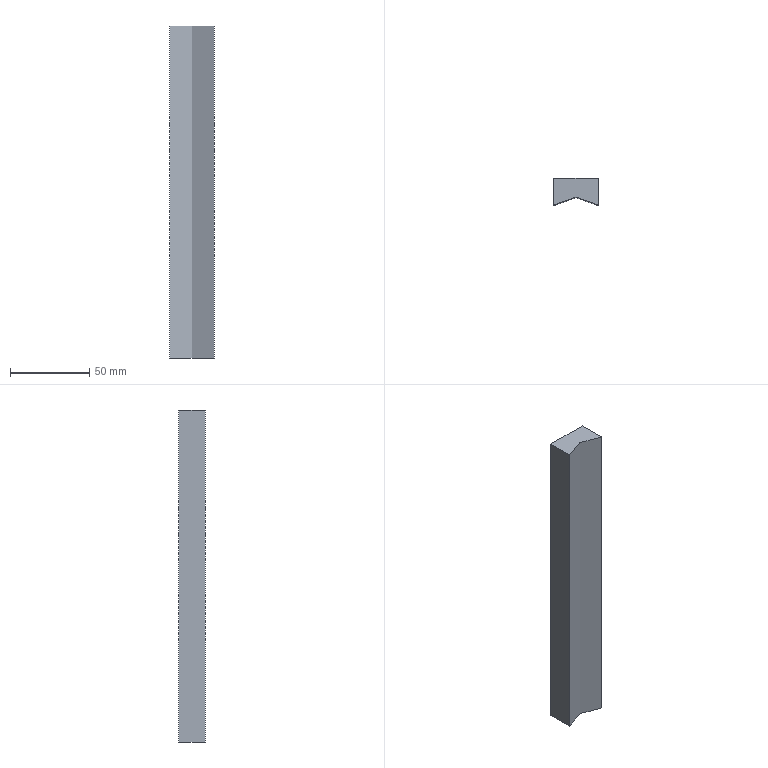Part | SolidWorks | features Extrusion 1 | 1 solid | 7 faces | box 28 x 17 x 210 mm | volume 85260 mm3 | plane 7
STEP:
#1=CARTESIAN_POINT('',(0.,0.,-105.));
#2=VERTEX_POINT('',#1);
#3=CARTESIAN_POINT('',(14.,-5.,-105.));
#4=VERTEX_POINT('',#3);
#5=CARTESIAN_POINT('',(14.,-5.,-105.));
#6=DIRECTION('',(0.9417,-0.3363,0.));
#7=VECTOR('',#6,1000.);
#8=LINE('',#5,#7);
#9=EDGE_CURVE('',#2,#4,#8,.T.);
#10=ORIENTED_EDGE('',*,*,#9,.T.);
#11=CARTESIAN_POINT('',(14.,-5.,105.));
#12=VERTEX_POINT('',#11);
#13=CARTESIAN_POINT('',(14.,-5.,105.));
#14=DIRECTION('',(0.,0.,-1.));
#15=VECTOR('',#14,1000.);
#16=LINE('',#13,#15);
#17=EDGE_CURVE('',#12,#4,#16,.T.);
#18=ORIENTED_EDGE('',*,*,#17,.F.);
#19=CARTESIAN_POINT('',(0.,0.,105.));
#20=VERTEX_POINT('',#19);
#21=CARTESIAN_POINT('',(14.,-5.,105.));
#22=DIRECTION('',(0.9417,-0.3363,0.));
#23=VECTOR('',#22,1000.);
#24=LINE('',#21,#23);
#25=EDGE_CURVE('',#20,#12,#24,.T.);
#26=ORIENTED_EDGE('',*,*,#25,.F.);
#27=CARTESIAN_POINT('',(0.,0.,105.));
#28=DIRECTION('',(0.,0.,-1.));
#29=VECTOR('',#28,1000.);
#30=LINE('',#27,#29);
#31=EDGE_CURVE('',#20,#2,#30,.T.);
#32=ORIENTED_EDGE('',*,*,#31,.T.);
#33=EDGE_LOOP('',(#10,#18,#26,#32));
#34=FACE_OUTER_BOUND('',#33,.T.);
#35=CARTESIAN_POINT('',(14.,-5.,105.));
#36=DIRECTION('',(0.3363,0.9417,0.));
#37=DIRECTION('',(-0.9417,0.3363,0.));
#38=AXIS2_PLACEMENT_3D('',#35,#36,#37);
#39=PLANE('',#38);
#40=ADVANCED_FACE('',(#34),#39,.F.);
#41=CARTESIAN_POINT('',(14.,12.,-105.));
#42=VERTEX_POINT('',#41);
#43=CARTESIAN_POINT('',(14.,12.,-105.));
#44=DIRECTION('',(0.,1.,0.));
#45=VECTOR('',#44,1000.);
#46=LINE('',#43,#45);
#47=EDGE_CURVE('',#4,#42,#46,.T.);
#48=ORIENTED_EDGE('',*,*,#47,.T.);
#49=CARTESIAN_POINT('',(14.,12.,105.));
#50=VERTEX_POINT('',#49);
#51=CARTESIAN_POINT('',(14.,12.,105.));
#52=DIRECTION('',(0.,0.,-1.));
#53=VECTOR('',#52,1000.);
#54=LINE('',#51,#53);
#55=EDGE_CURVE('',#50,#42,#54,.T.);
#56=ORIENTED_EDGE('',*,*,#55,.F.);
#57=CARTESIAN_POINT('',(14.,12.,105.));
#58=DIRECTION('',(0.,1.,0.));
#59=VECTOR('',#58,1000.);
#60=LINE('',#57,#59);
#61=EDGE_CURVE('',#12,#50,#60,.T.);
#62=ORIENTED_EDGE('',*,*,#61,.F.);
#63=ORIENTED_EDGE('',*,*,#17,.T.);
#64=EDGE_LOOP('',(#48,#56,#62,#63));
#65=FACE_OUTER_BOUND('',#64,.T.);
#66=CARTESIAN_POINT('',(14.,12.,105.));
#67=DIRECTION('',(-1.,0.,0.));
#68=DIRECTION('',(0.,0.,1.));
#69=AXIS2_PLACEMENT_3D('',#66,#67,#68);
#70=PLANE('',#69);
#71=ADVANCED_FACE('',(#65),#70,.F.);
#72=CARTESIAN_POINT('',(-14.,12.,-105.));
#73=VERTEX_POINT('',#72);
#74=CARTESIAN_POINT('',(-14.,12.,-105.));
#75=DIRECTION('',(-1.,0.,0.));
#76=VECTOR('',#75,1000.);
#77=LINE('',#74,#76);
#78=EDGE_CURVE('',#42,#73,#77,.T.);
#79=ORIENTED_EDGE('',*,*,#78,.T.);
#80=CARTESIAN_POINT('',(-14.,12.,105.));
#81=VERTEX_POINT('',#80);
#82=CARTESIAN_POINT('',(-14.,12.,105.));
#83=DIRECTION('',(0.,0.,-1.));
#84=VECTOR('',#83,1000.);
#85=LINE('',#82,#84);
#86=EDGE_CURVE('',#81,#73,#85,.T.);
#87=ORIENTED_EDGE('',*,*,#86,.F.);
#88=CARTESIAN_POINT('',(-14.,12.,105.));
#89=DIRECTION('',(-1.,0.,0.));
#90=VECTOR('',#89,1000.);
#91=LINE('',#88,#90);
#92=EDGE_CURVE('',#50,#81,#91,.T.);
#93=ORIENTED_EDGE('',*,*,#92,.F.);
#94=ORIENTED_EDGE('',*,*,#55,.T.);
#95=EDGE_LOOP('',(#79,#87,#93,#94));
#96=FACE_OUTER_BOUND('',#95,.T.);
#97=CARTESIAN_POINT('',(-14.,12.,105.));
#98=DIRECTION('',(0.,-1.,0.));
#99=DIRECTION('',(0.,0.,-1.));
#100=AXIS2_PLACEMENT_3D('',#97,#98,#99);
#101=PLANE('',#100);
#102=ADVANCED_FACE('',(#96),#101,.F.);
#103=CARTESIAN_POINT('',(-14.,-5.,-105.));
#104=VERTEX_POINT('',#103);
#105=CARTESIAN_POINT('',(-14.,-5.,-105.));
#106=DIRECTION('',(0.,-1.,0.));
#107=VECTOR('',#106,1000.);
#108=LINE('',#105,#107);
#109=EDGE_CURVE('',#73,#104,#108,.T.);
#110=ORIENTED_EDGE('',*,*,#109,.T.);
#111=CARTESIAN_POINT('',(-14.,-5.,105.));
#112=VERTEX_POINT('',#111);
#113=CARTESIAN_POINT('',(-14.,-5.,105.));
#114=DIRECTION('',(0.,0.,-1.));
#115=VECTOR('',#114,1000.);
#116=LINE('',#113,#115);
#117=EDGE_CURVE('',#112,#104,#116,.T.);
#118=ORIENTED_EDGE('',*,*,#117,.F.);
#119=CARTESIAN_POINT('',(-14.,-5.,105.));
#120=DIRECTION('',(0.,-1.,0.));
#121=VECTOR('',#120,1000.);
#122=LINE('',#119,#121);
#123=EDGE_CURVE('',#81,#112,#122,.T.);
#124=ORIENTED_EDGE('',*,*,#123,.F.);
#125=ORIENTED_EDGE('',*,*,#86,.T.);
#126=EDGE_LOOP('',(#110,#118,#124,#125));
#127=FACE_OUTER_BOUND('',#126,.T.);
#128=CARTESIAN_POINT('',(-14.,-5.,105.));
#129=DIRECTION('',(1.,0.,0.));
#130=DIRECTION('',(0.,0.,-1.));
#131=AXIS2_PLACEMENT_3D('',#128,#129,#130);
#132=PLANE('',#131);
#133=ADVANCED_FACE('',(#127),#132,.F.);
#134=CARTESIAN_POINT('',(0.,0.,-105.));
#135=DIRECTION('',(0.9417,0.3363,0.));
#136=VECTOR('',#135,1000.);
#137=LINE('',#134,#136);
#138=EDGE_CURVE('',#104,#2,#137,.T.);
#139=ORIENTED_EDGE('',*,*,#138,.T.);
#140=ORIENTED_EDGE('',*,*,#31,.F.);
#141=CARTESIAN_POINT('',(0.,0.,105.));
#142=DIRECTION('',(0.9417,0.3363,0.));
#143=VECTOR('',#142,1000.);
#144=LINE('',#141,#143);
#145=EDGE_CURVE('',#112,#20,#144,.T.);
#146=ORIENTED_EDGE('',*,*,#145,.F.);
#147=ORIENTED_EDGE('',*,*,#117,.T.);
#148=EDGE_LOOP('',(#139,#140,#146,#147));
#149=FACE_OUTER_BOUND('',#148,.T.);
#150=CARTESIAN_POINT('',(0.,0.,105.));
#151=DIRECTION('',(-0.3363,0.9417,0.));
#152=DIRECTION('',(-0.9417,-0.3363,0.));
#153=AXIS2_PLACEMENT_3D('',#150,#151,#152);
#154=PLANE('',#153);
#155=ADVANCED_FACE('',(#149),#154,.F.);
#156=ORIENTED_EDGE('',*,*,#25,.T.);
#157=ORIENTED_EDGE('',*,*,#61,.T.);
#158=ORIENTED_EDGE('',*,*,#92,.T.);
#159=ORIENTED_EDGE('',*,*,#123,.T.);
#160=ORIENTED_EDGE('',*,*,#145,.T.);
#161=EDGE_LOOP('',(#156,#157,#158,#159,#160));
#162=FACE_OUTER_BOUND('',#161,.T.);
#163=CARTESIAN_POINT('',(0.,0.,105.));
#164=DIRECTION('',(0.,0.,-1.));
#165=DIRECTION('',(-1.,0.,0.));
#166=AXIS2_PLACEMENT_3D('',#163,#164,#165);
#167=PLANE('',#166);
#168=ADVANCED_FACE('',(#162),#167,.F.);
#169=ORIENTED_EDGE('',*,*,#9,.F.);
#170=ORIENTED_EDGE('',*,*,#138,.F.);
#171=ORIENTED_EDGE('',*,*,#109,.F.);
#172=ORIENTED_EDGE('',*,*,#78,.F.);
#173=ORIENTED_EDGE('',*,*,#47,.F.);
#174=EDGE_LOOP('',(#169,#170,#171,#172,#173));
#175=FACE_OUTER_BOUND('',#174,.T.);
#176=CARTESIAN_POINT('',(0.,0.,-105.));
#177=DIRECTION('',(0.,0.,-1.));
#178=DIRECTION('',(-1.,0.,0.));
#179=AXIS2_PLACEMENT_3D('',#176,#177,#178);
#180=PLANE('',#179);
#181=ADVANCED_FACE('',(#175),#180,.T.);
#182=CLOSED_SHELL('',(#40,#71,#102,#133,#155,#168,#181));
#183=MANIFOLD_SOLID_BREP('',#182);
#184=CARTESIAN_POINT('',(0.,0.,0.));
#185=DIRECTION('',(0.,0.,1.));
#186=DIRECTION('',(1.,0.,0.));
#187=AXIS2_PLACEMENT_3D('',#184,#185,#186);
#188=(LENGTH_UNIT()NAMED_UNIT(*)SI_UNIT(.MILLI.,.METRE.));
#189=UNCERTAINTY_MEASURE_WITH_UNIT(LENGTH_MEASURE(0.00001),#188,'','');
#190=(NAMED_UNIT(*)PLANE_ANGLE_UNIT()SI_UNIT($,.RADIAN.));
#191=(NAMED_UNIT(*)SI_UNIT($,.STERADIAN.)SOLID_ANGLE_UNIT());
#192=(GEOMETRIC_REPRESENTATION_CONTEXT(3)GLOBAL_UNCERTAINTY_ASSIGNED_CONTEXT((#189))GLOBAL_UNIT_ASSIGNED_CONTEXT((#188,#190,#191))REPRESENTATION_CONTEXT('',''));
#193=ADVANCED_BREP_SHAPE_REPRESENTATION('',(#183,#187),#192);